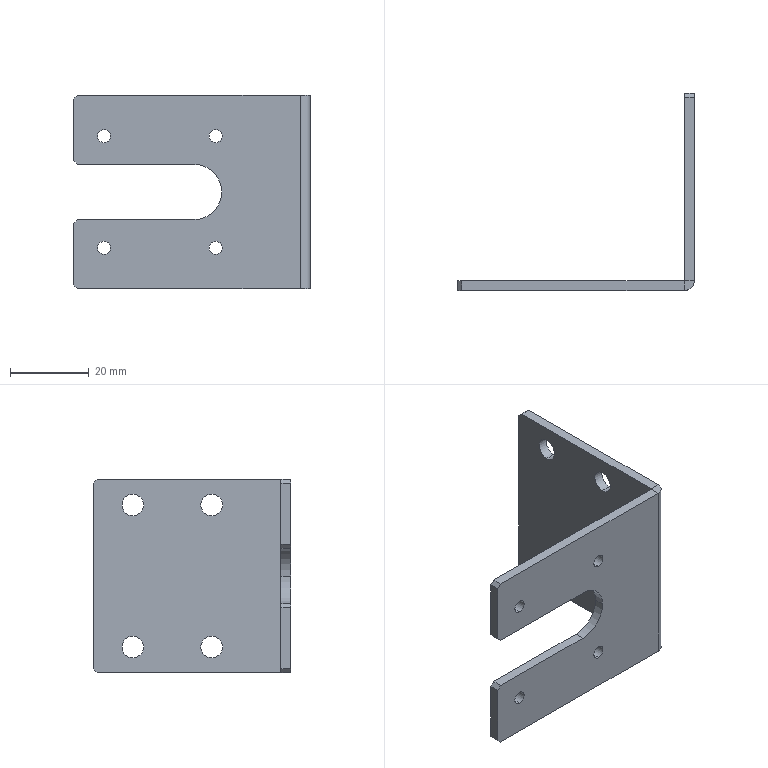Part | STEP file | 1 solid | 41 faces | box 60 x 50 x 49 mm | volume 11507 mm3 | plane 21 | cylinder 20 | commonest cylinder face diameters 3.3 x8 5.5 x8 14 x2 0.2 x1 5.2 x1